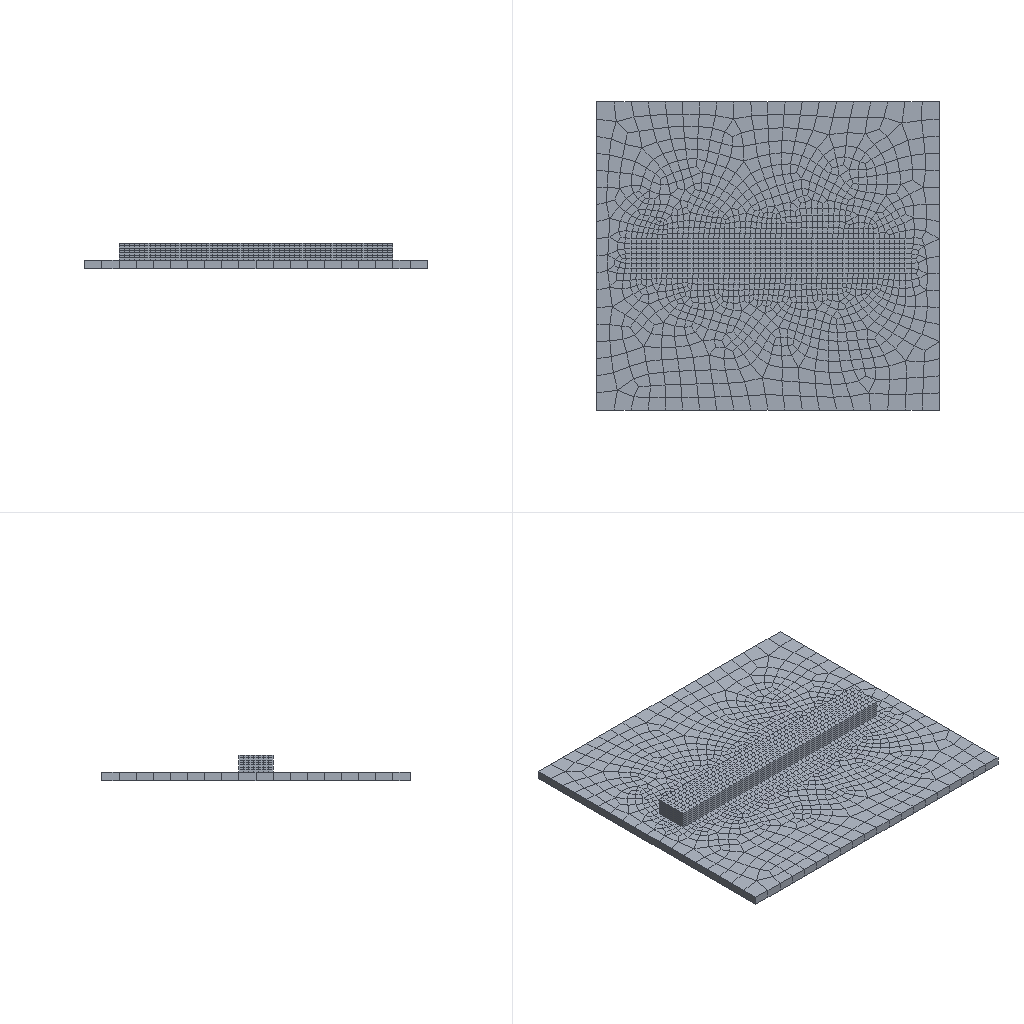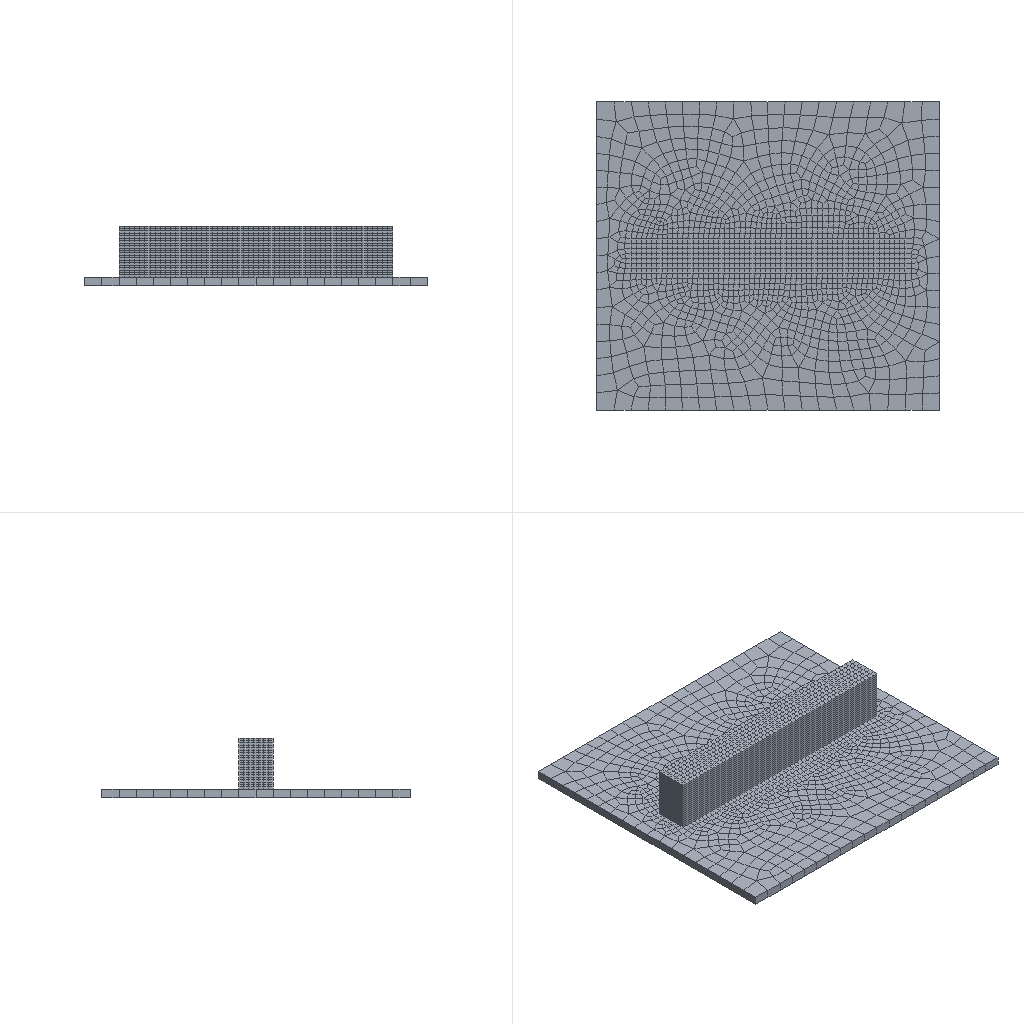Simulation study | abaqus
Set-up summary:
category,name,step,type,value,unit,region
solver,abaqus
solver,version,,,Abaqus/Standard 3DEXPERIENCE R2017x
solver,version,,,Abaqus/Standard 3DEXPERIENCE R2017x
units,not stated in the deck,,not stated
analysis,deck1,,coupled temperature-displacement,coupled temperature-displacement
load_step,Step-1,Step-1,coupled temperature-displacement,nlgeom=True
load_step,Step-2,Step-2,coupled temperature-displacement,nlgeom=True
contact,interactions,,,general=0 pairs=0 ties=0
load_step,requested,,,2
mesh,nodes,,,6270
mesh,elements,,,4181
element_type,C3D8RT,,solid,4181
load,load commands in deck,,count,1
bc,support commands in deck,,count,1
analysis,deck2,,coupled temperature-displacement,coupled temperature-displacement
load_step,Step-1,Step-1,coupled temperature-displacement,nlgeom=True
load_step,Step-2,Step-2,coupled temperature-displacement,nlgeom=True
load_step,Step-3,Step-3,coupled temperature-displacement,nlgeom=True
load_step,Step-4,Step-4,coupled temperature-displacement,nlgeom=True
contact,interactions,,,general=0 pairs=0 ties=0
load_step,requested,,,4
mesh,nodes,,,12318
mesh,elements,,,9375
element_type,C3D8RT,,solid,9375
load,load commands in deck,,count,1
bc,support commands in deck,,count,1
material,MATERIAL-1,,in results
material,MATERIAL-1,,in results
check,setup vs results,,match,"per instance, exact: element labels, types and connectivity; labels of the nodes the elements use; coordinates of those nodes at SINGLE_PRECISION in 1 of 1 instance(s)"
check,setup vs results,,match,"per instance, exact: element labels, types and connectivity; labels of the nodes the elements use; coordinates of those nodes at SINGLE_PRECISION in 1 of 1 instance(s)"
Results summary:
result,step,,completed,increments=6 time=0.01/0.01
result,step,,completed,increments=24 time=10.0/10.0
result,analysis,,,"coupled temperature-displacement, steady state"
result,last_loadstep,,,2
result,analysis steps,,count,2
result,primary field,,,"U, NT11"
result,reaction total,,FX,-1.24,model units
result,reaction total,,FY,0.001949,model units
result,reaction total,,FZ,7.339,model units
result,step,,completed,increments=6 time=0.01/0.01
result,step,,completed,increments=24 time=10.0/10.0
result,step,,completed,increments=24 time=10.0/10.0
result,step,,completed,increments=24 time=10.0/10.0
result,analysis,,,"coupled temperature-displacement, steady state"
result,last_loadstep,,,4
result,analysis steps,,count,4
result,primary field,,,"U, NT11"
result,reaction total,,FX,-2.409,model units
result,reaction total,,FY,-0.004641,model units
result,reaction total,,FZ,13.669,model units